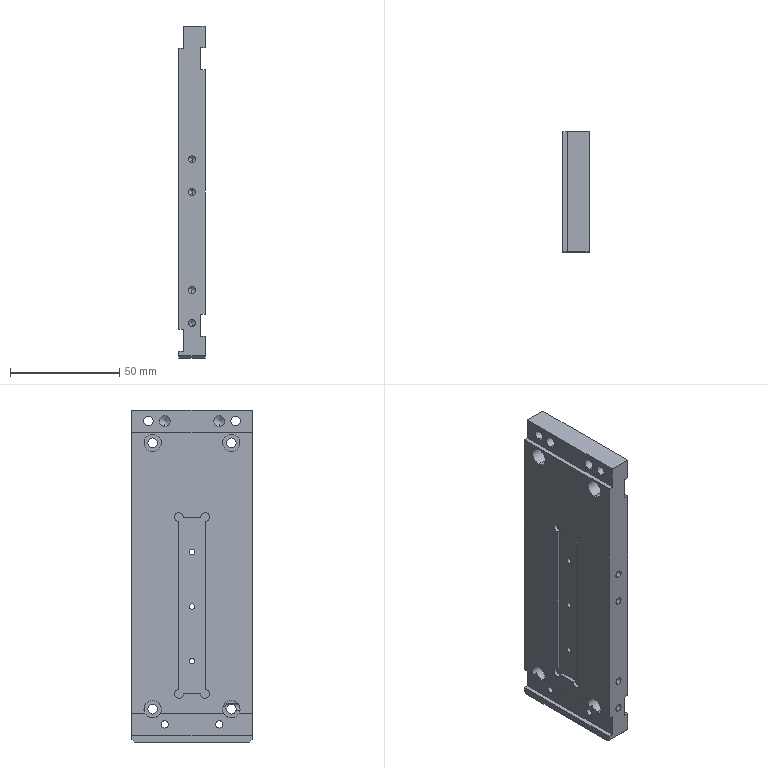Part | SolidWorks | features HoleWzd 6, ICE 5, MirrorPattern 2, Chamfer 1, Cut 1, Extrusion 1 | 1 solid | 100 faces | box 12 x 55 x 152 mm | volume 91517 mm3 | cylinder 52 | plane 33 | cone 15 | commonest cylinder face diameters 3.3 x16 4.4 x8 8 x8 2.5 x6 4 x6 4.5 x4